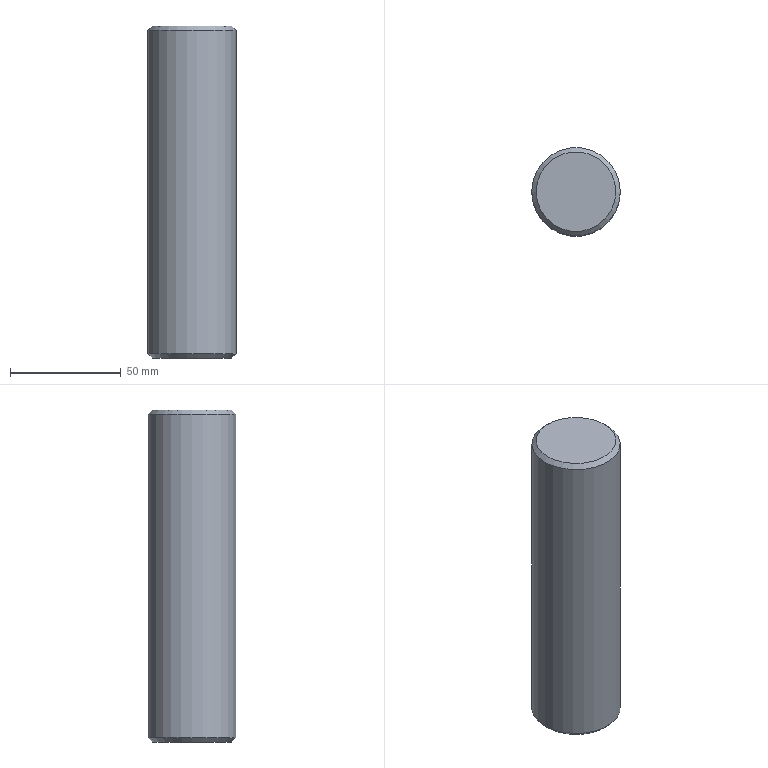Part | STEP file | P011002NM11-000 | 1 solid | 73 faces | box 40 x 40 x 150 mm | volume 185820 mm3 | plane 44 | other 14 | cone 8 | cylinder 7 | commonest cylinder face diameters 10.18 x3 10.2 x1 11.8 x1 12 x1 40 x1